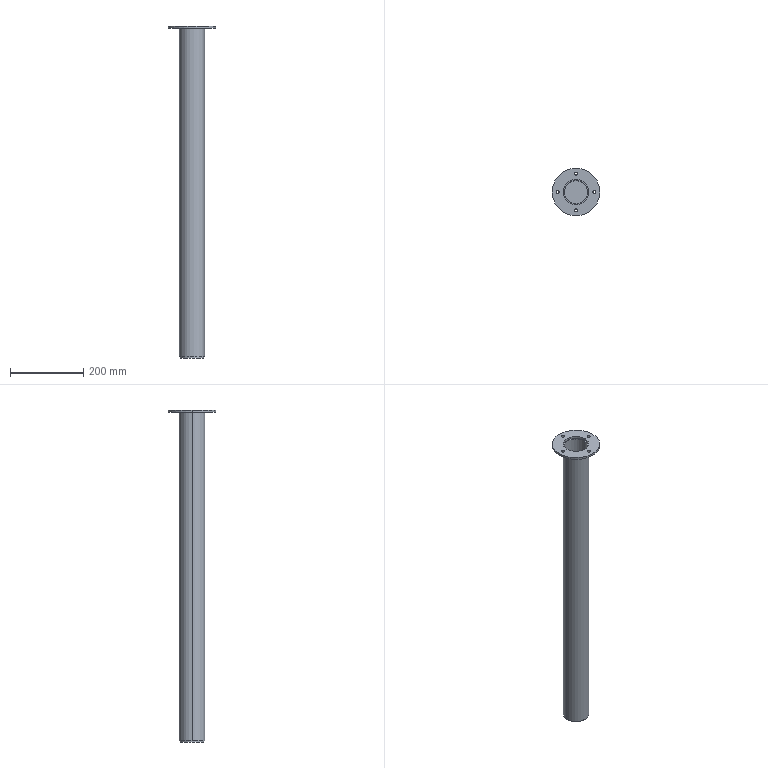Part | SolidWorks | features ICE 2, ExtruThin 1, HoleWzd 1 | 3 solids | 24 faces | box 130 x 130 x 909 mm | volume 633307 mm3 | cylinder 18 | plane 6 | commonest cylinder face diameters 8 x8 64 x4 70 x4 130 x2
STEP:
#1=CARTESIAN_POINT('',(-32.,0.,900.));
#2=VERTEX_POINT('',#1);
#3=CARTESIAN_POINT('',(32.,0.,900.));
#4=VERTEX_POINT('',#3);
#5=CARTESIAN_POINT('',(0.,0.,900.));
#6=DIRECTION('',(0.,0.,1.));
#7=DIRECTION('',(1.,0.,0.));
#8=AXIS2_PLACEMENT_3D('',#5,#6,#7);
#9=CIRCLE('',#8,32.);
#10=EDGE_CURVE('',#2,#4,#9,.T.);
#11=ORIENTED_EDGE('',*,*,#10,.T.);
#12=CARTESIAN_POINT('',(32.,0.,0.));
#13=VERTEX_POINT('',#12);
#14=CARTESIAN_POINT('',(32.,0.,900.));
#15=DIRECTION('',(0.,0.,-1.));
#16=VECTOR('',#15,1000.);
#17=LINE('',#14,#16);
#18=EDGE_CURVE('',#4,#13,#17,.T.);
#19=ORIENTED_EDGE('',*,*,#18,.T.);
#20=CARTESIAN_POINT('',(-32.,0.,0.));
#21=VERTEX_POINT('',#20);
#22=CARTESIAN_POINT('',(0.,0.,0.));
#23=DIRECTION('',(0.,0.,1.));
#24=DIRECTION('',(1.,0.,0.));
#25=AXIS2_PLACEMENT_3D('',#22,#23,#24);
#26=CIRCLE('',#25,32.);
#27=EDGE_CURVE('',#21,#13,#26,.T.);
#28=ORIENTED_EDGE('',*,*,#27,.F.);
#29=CARTESIAN_POINT('',(-32.,0.,900.));
#30=DIRECTION('',(0.,0.,-1.));
#31=VECTOR('',#30,1000.);
#32=LINE('',#29,#31);
#33=EDGE_CURVE('',#2,#21,#32,.T.);
#34=ORIENTED_EDGE('',*,*,#33,.F.);
#35=EDGE_LOOP('',(#11,#19,#28,#34));
#36=FACE_OUTER_BOUND('',#35,.T.);
#37=CARTESIAN_POINT('',(0.,0.,900.));
#38=DIRECTION('',(0.,0.,-1.));
#39=DIRECTION('',(-1.,0.,0.));
#40=AXIS2_PLACEMENT_3D('',#37,#38,#39);
#41=CYLINDRICAL_SURFACE('',#40,32.);
#42=ADVANCED_FACE('',(#36),#41,.F.);
#43=CARTESIAN_POINT('',(35.,0.,900.));
#44=VERTEX_POINT('',#43);
#45=CARTESIAN_POINT('',(-35.,0.,900.));
#46=VERTEX_POINT('',#45);
#47=CARTESIAN_POINT('',(0.,0.,900.));
#48=DIRECTION('',(0.,0.,1.));
#49=DIRECTION('',(1.,0.,0.));
#50=AXIS2_PLACEMENT_3D('',#47,#48,#49);
#51=CIRCLE('',#50,35.);
#52=EDGE_CURVE('',#44,#46,#51,.T.);
#53=ORIENTED_EDGE('',*,*,#52,.F.);
#54=CARTESIAN_POINT('',(35.,0.,0.));
#55=VERTEX_POINT('',#54);
#56=CARTESIAN_POINT('',(35.,0.,900.));
#57=DIRECTION('',(0.,0.,-1.));
#58=VECTOR('',#57,1000.);
#59=LINE('',#56,#58);
#60=EDGE_CURVE('',#44,#55,#59,.T.);
#61=ORIENTED_EDGE('',*,*,#60,.T.);
#62=CARTESIAN_POINT('',(-35.,0.,0.));
#63=VERTEX_POINT('',#62);
#64=CARTESIAN_POINT('',(0.,0.,0.));
#65=DIRECTION('',(0.,0.,1.));
#66=DIRECTION('',(1.,0.,0.));
#67=AXIS2_PLACEMENT_3D('',#64,#65,#66);
#68=CIRCLE('',#67,35.);
#69=EDGE_CURVE('',#55,#63,#68,.T.);
#70=ORIENTED_EDGE('',*,*,#69,.T.);
#71=CARTESIAN_POINT('',(-35.,0.,900.));
#72=DIRECTION('',(0.,0.,-1.));
#73=VECTOR('',#72,1000.);
#74=LINE('',#71,#73);
#75=EDGE_CURVE('',#46,#63,#74,.T.);
#76=ORIENTED_EDGE('',*,*,#75,.F.);
#77=EDGE_LOOP('',(#53,#61,#70,#76));
#78=FACE_OUTER_BOUND('',#77,.T.);
#79=CARTESIAN_POINT('',(0.,0.,900.));
#80=DIRECTION('',(0.,0.,-1.));
#81=DIRECTION('',(-1.,0.,0.));
#82=AXIS2_PLACEMENT_3D('',#79,#80,#81);
#83=CYLINDRICAL_SURFACE('',#82,35.);
#84=ADVANCED_FACE('',(#78),#83,.T.);
#85=CARTESIAN_POINT('',(0.,0.,900.));
#86=DIRECTION('',(0.,0.,1.));
#87=DIRECTION('',(1.,0.,0.));
#88=AXIS2_PLACEMENT_3D('',#85,#86,#87);
#89=CIRCLE('',#88,35.);
#90=EDGE_CURVE('',#46,#44,#89,.T.);
#91=ORIENTED_EDGE('',*,*,#90,.T.);
#92=ORIENTED_EDGE('',*,*,#52,.T.);
#93=EDGE_LOOP('',(#91,#92));
#94=FACE_OUTER_BOUND('',#93,.T.);
#95=ORIENTED_EDGE('',*,*,#10,.F.);
#96=CARTESIAN_POINT('',(0.,0.,900.));
#97=DIRECTION('',(0.,0.,1.));
#98=DIRECTION('',(1.,0.,0.));
#99=AXIS2_PLACEMENT_3D('',#96,#97,#98);
#100=CIRCLE('',#99,32.);
#101=EDGE_CURVE('',#4,#2,#100,.T.);
#102=ORIENTED_EDGE('',*,*,#101,.F.);
#103=EDGE_LOOP('',(#95,#102));
#104=FACE_BOUND('',#103,.T.);
#105=CARTESIAN_POINT('',(0.,0.,900.));
#106=DIRECTION('',(0.,0.,1.));
#107=DIRECTION('',(1.,0.,0.));
#108=AXIS2_PLACEMENT_3D('',#105,#106,#107);
#109=PLANE('',#108);
#110=ADVANCED_FACE('',(#94,#104),#109,.T.);
#111=CARTESIAN_POINT('',(0.,0.,0.));
#112=DIRECTION('',(0.,0.,1.));
#113=DIRECTION('',(1.,0.,0.));
#114=AXIS2_PLACEMENT_3D('',#111,#112,#113);
#115=CIRCLE('',#114,35.);
#116=EDGE_CURVE('',#63,#55,#115,.T.);
#117=ORIENTED_EDGE('',*,*,#116,.F.);
#118=ORIENTED_EDGE('',*,*,#69,.F.);
#119=EDGE_LOOP('',(#117,#118));
#120=FACE_OUTER_BOUND('',#119,.T.);
#121=ORIENTED_EDGE('',*,*,#27,.T.);
#122=CARTESIAN_POINT('',(0.,0.,0.));
#123=DIRECTION('',(0.,0.,1.));
#124=DIRECTION('',(1.,0.,0.));
#125=AXIS2_PLACEMENT_3D('',#122,#123,#124);
#126=CIRCLE('',#125,32.);
#127=EDGE_CURVE('',#13,#21,#126,.T.);
#128=ORIENTED_EDGE('',*,*,#127,.T.);
#129=EDGE_LOOP('',(#121,#128));
#130=FACE_BOUND('',#129,.T.);
#131=CARTESIAN_POINT('',(0.,0.,0.));
#132=DIRECTION('',(0.,0.,1.));
#133=DIRECTION('',(1.,0.,0.));
#134=AXIS2_PLACEMENT_3D('',#131,#132,#133);
#135=PLANE('',#134);
#136=ADVANCED_FACE('',(#120,#130),#135,.F.);
#137=ORIENTED_EDGE('',*,*,#60,.F.);
#138=ORIENTED_EDGE('',*,*,#90,.F.);
#139=ORIENTED_EDGE('',*,*,#75,.T.);
#140=ORIENTED_EDGE('',*,*,#116,.T.);
#141=EDGE_LOOP('',(#137,#138,#139,#140));
#142=FACE_OUTER_BOUND('',#141,.T.);
#143=CARTESIAN_POINT('',(0.,0.,900.));
#144=DIRECTION('',(0.,0.,-1.));
#145=DIRECTION('',(-1.,0.,0.));
#146=AXIS2_PLACEMENT_3D('',#143,#144,#145);
#147=CYLINDRICAL_SURFACE('',#146,35.);
#148=ADVANCED_FACE('',(#142),#147,.T.);
#149=ORIENTED_EDGE('',*,*,#18,.F.);
#150=ORIENTED_EDGE('',*,*,#101,.T.);
#151=ORIENTED_EDGE('',*,*,#33,.T.);
#152=ORIENTED_EDGE('',*,*,#127,.F.);
#153=EDGE_LOOP('',(#149,#150,#151,#152));
#154=FACE_OUTER_BOUND('',#153,.T.);
#155=CARTESIAN_POINT('',(0.,0.,900.));
#156=DIRECTION('',(0.,0.,-1.));
#157=DIRECTION('',(-1.,0.,0.));
#158=AXIS2_PLACEMENT_3D('',#155,#156,#157);
#159=CYLINDRICAL_SURFACE('',#158,32.);
#160=ADVANCED_FACE('',(#154),#159,.F.);
#161=CLOSED_SHELL('',(#42,#84,#110,#136,#148,#160));
#162=MANIFOLD_SOLID_BREP('',#161);
#163=CARTESIAN_POINT('',(-32.,0.,-3.));
#164=VERTEX_POINT('',#163);
#165=CARTESIAN_POINT('',(32.,0.,-3.));
#166=VERTEX_POINT('',#165);
#167=CARTESIAN_POINT('',(0.,0.,-3.));
#168=DIRECTION('',(0.,0.,-1.));
#169=DIRECTION('',(-1.,0.,0.));
#170=AXIS2_PLACEMENT_3D('',#167,#168,#169);
#171=CIRCLE('',#170,32.);
#172=EDGE_CURVE('',#164,#166,#171,.T.);
#173=ORIENTED_EDGE('',*,*,#172,.F.);
#174=CARTESIAN_POINT('',(-32.,0.,0.));
#175=VERTEX_POINT('',#174);
#176=CARTESIAN_POINT('',(-32.,0.,-3.));
#177=DIRECTION('',(0.,0.,1.));
#178=VECTOR('',#177,1000.);
#179=LINE('',#176,#178);
#180=EDGE_CURVE('',#164,#175,#179,.T.);
#181=ORIENTED_EDGE('',*,*,#180,.T.);
#182=CARTESIAN_POINT('',(32.,0.,0.));
#183=VERTEX_POINT('',#182);
#184=CARTESIAN_POINT('',(0.,0.,0.));
#185=DIRECTION('',(0.,0.,-1.));
#186=DIRECTION('',(-1.,0.,0.));
#187=AXIS2_PLACEMENT_3D('',#184,#185,#186);
#188=CIRCLE('',#187,32.);
#189=EDGE_CURVE('',#175,#183,#188,.T.);
#190=ORIENTED_EDGE('',*,*,#189,.T.);
#191=CARTESIAN_POINT('',(32.,0.,-3.));
#192=DIRECTION('',(0.,0.,1.));
#193=VECTOR('',#192,1000.);
#194=LINE('',#191,#193);
#195=EDGE_CURVE('',#166,#183,#194,.T.);
#196=ORIENTED_EDGE('',*,*,#195,.F.);
#197=EDGE_LOOP('',(#173,#181,#190,#196));
#198=FACE_OUTER_BOUND('',#197,.T.);
#199=CARTESIAN_POINT('',(0.,0.,-3.));
#200=DIRECTION('',(0.,0.,1.));
#201=DIRECTION('',(1.,0.,0.));
#202=AXIS2_PLACEMENT_3D('',#199,#200,#201);
#203=CYLINDRICAL_SURFACE('',#202,32.);
#204=ADVANCED_FACE('',(#198),#203,.T.);
#205=ORIENTED_EDGE('',*,*,#180,.F.);
#206=CARTESIAN_POINT('',(0.,0.,-3.));
#207=DIRECTION('',(0.,0.,-1.));
#208=DIRECTION('',(-1.,0.,0.));
#209=AXIS2_PLACEMENT_3D('',#206,#207,#208);
#210=CIRCLE('',#209,32.);
#211=EDGE_CURVE('',#166,#164,#210,.T.);
#212=ORIENTED_EDGE('',*,*,#211,.F.);
#213=ORIENTED_EDGE('',*,*,#195,.T.);
#214=CARTESIAN_POINT('',(0.,0.,0.));
#215=DIRECTION('',(0.,0.,-1.));
#216=DIRECTION('',(-1.,0.,0.));
#217=AXIS2_PLACEMENT_3D('',#214,#215,#216);
#218=CIRCLE('',#217,32.);
#219=EDGE_CURVE('',#183,#175,#218,.T.);
#220=ORIENTED_EDGE('',*,*,#219,.T.);
#221=EDGE_LOOP('',(#205,#212,#213,#220));
#222=FACE_OUTER_BOUND('',#221,.T.);
#223=CARTESIAN_POINT('',(0.,0.,-3.));
#224=DIRECTION('',(0.,0.,1.));
#225=DIRECTION('',(1.,0.,0.));
#226=AXIS2_PLACEMENT_3D('',#223,#224,#225);
#227=CYLINDRICAL_SURFACE('',#226,32.);
#228=ADVANCED_FACE('',(#222),#227,.T.);
#229=ORIENTED_EDGE('',*,*,#211,.T.);
#230=ORIENTED_EDGE('',*,*,#172,.T.);
#231=EDGE_LOOP('',(#229,#230));
#232=FACE_OUTER_BOUND('',#231,.T.);
#233=CARTESIAN_POINT('',(0.,0.,-3.));
#234=DIRECTION('',(0.,0.,-1.));
#235=DIRECTION('',(-1.,0.,0.));
#236=AXIS2_PLACEMENT_3D('',#233,#234,#235);
#237=PLANE('',#236);
#238=ADVANCED_FACE('',(#232),#237,.T.);
#239=ORIENTED_EDGE('',*,*,#219,.F.);
#240=ORIENTED_EDGE('',*,*,#189,.F.);
#241=EDGE_LOOP('',(#239,#240));
#242=FACE_OUTER_BOUND('',#241,.T.);
#243=CARTESIAN_POINT('',(0.,0.,0.));
#244=DIRECTION('',(0.,0.,-1.));
#245=DIRECTION('',(-1.,0.,0.));
#246=AXIS2_PLACEMENT_3D('',#243,#244,#245);
#247=PLANE('',#246);
#248=ADVANCED_FACE('',(#242),#247,.F.);
#249=CLOSED_SHELL('',(#204,#228,#238,#248));
#250=MANIFOLD_SOLID_BREP('',#249);
#251=CARTESIAN_POINT('',(-4.,50.,900.));
#252=VERTEX_POINT('',#251);
#253=CARTESIAN_POINT('',(4.,50.,900.));
#254=VERTEX_POINT('',#253);
#255=CARTESIAN_POINT('',(0.,50.,900.));
#256=DIRECTION('',(0.,0.,1.));
#257=DIRECTION('',(1.,0.,0.));
#258=AXIS2_PLACEMENT_3D('',#255,#256,#257);
#259=CIRCLE('',#258,4.);
#260=EDGE_CURVE('',#252,#254,#259,.T.);
#261=ORIENTED_EDGE('',*,*,#260,.F.);
#262=CARTESIAN_POINT('',(-4.,50.,906.));
#263=VERTEX_POINT('',#262);
#264=CARTESIAN_POINT('',(-4.,50.,906.));
#265=DIRECTION('',(0.,0.,1.));
#266=VECTOR('',#265,1000.);
#267=LINE('',#264,#266);
#268=EDGE_CURVE('',#252,#263,#267,.T.);
#269=ORIENTED_EDGE('',*,*,#268,.T.);
#270=CARTESIAN_POINT('',(4.,50.,906.));
#271=VERTEX_POINT('',#270);
#272=CARTESIAN_POINT('',(0.,50.,906.));
#273=DIRECTION('',(0.,0.,1.));
#274=DIRECTION('',(1.,0.,0.));
#275=AXIS2_PLACEMENT_3D('',#272,#273,#274);
#276=CIRCLE('',#275,4.);
#277=EDGE_CURVE('',#263,#271,#276,.T.);
#278=ORIENTED_EDGE('',*,*,#277,.T.);
#279=CARTESIAN_POINT('',(4.,50.,906.));
#280=DIRECTION('',(0.,0.,1.));
#281=VECTOR('',#280,1000.);
#282=LINE('',#279,#281);
#283=EDGE_CURVE('',#254,#271,#282,.T.);
#284=ORIENTED_EDGE('',*,*,#283,.F.);
#285=EDGE_LOOP('',(#261,#269,#278,#284));
#286=FACE_OUTER_BOUND('',#285,.T.);
#287=CARTESIAN_POINT('',(0.,50.,906.));
#288=DIRECTION('',(0.,0.,1.));
#289=DIRECTION('',(1.,0.,0.));
#290=AXIS2_PLACEMENT_3D('',#287,#288,#289);
#291=CYLINDRICAL_SURFACE('',#290,4.);
#292=ADVANCED_FACE('',(#286),#291,.F.);
#293=CARTESIAN_POINT('',(-54.,0.,900.));
#294=VERTEX_POINT('',#293);
#295=CARTESIAN_POINT('',(-46.,0.,900.));
#296=VERTEX_POINT('',#295);
#297=CARTESIAN_POINT('',(-50.,0.,900.));
#298=DIRECTION('',(0.,0.,1.));
#299=DIRECTION('',(1.,0.,0.));
#300=AXIS2_PLACEMENT_3D('',#297,#298,#299);
#301=CIRCLE('',#300,4.);
#302=EDGE_CURVE('',#294,#296,#301,.T.);
#303=ORIENTED_EDGE('',*,*,#302,.F.);
#304=CARTESIAN_POINT('',(-54.,0.,906.));
#305=VERTEX_POINT('',#304);
#306=CARTESIAN_POINT('',(-54.,0.,906.));
#307=DIRECTION('',(0.,0.,1.));
#308=VECTOR('',#307,1000.);
#309=LINE('',#306,#308);
#310=EDGE_CURVE('',#294,#305,#309,.T.);
#311=ORIENTED_EDGE('',*,*,#310,.T.);
#312=CARTESIAN_POINT('',(-46.,0.,906.));
#313=VERTEX_POINT('',#312);
#314=CARTESIAN_POINT('',(-50.,0.,906.));
#315=DIRECTION('',(0.,0.,1.));
#316=DIRECTION('',(1.,0.,0.));
#317=AXIS2_PLACEMENT_3D('',#314,#315,#316);
#318=CIRCLE('',#317,4.);
#319=EDGE_CURVE('',#305,#313,#318,.T.);
#320=ORIENTED_EDGE('',*,*,#319,.T.);
#321=CARTESIAN_POINT('',(-46.,0.,906.));
#322=DIRECTION('',(0.,0.,1.));
#323=VECTOR('',#322,1000.);
#324=LINE('',#321,#323);
#325=EDGE_CURVE('',#296,#313,#324,.T.);
#326=ORIENTED_EDGE('',*,*,#325,.F.);
#327=EDGE_LOOP('',(#303,#311,#320,#326));
#328=FACE_OUTER_BOUND('',#327,.T.);
#329=CARTESIAN_POINT('',(-50.,0.,906.));
#330=DIRECTION('',(0.,0.,1.));
#331=DIRECTION('',(1.,0.,0.));
#332=AXIS2_PLACEMENT_3D('',#329,#330,#331);
#333=CYLINDRICAL_SURFACE('',#332,4.);
#334=ADVANCED_FACE('',(#328),#333,.F.);
#335=CARTESIAN_POINT('',(-4.,-50.,900.));
#336=VERTEX_POINT('',#335);
#337=CARTESIAN_POINT('',(4.,-50.,900.));
#338=VERTEX_POINT('',#337);
#339=CARTESIAN_POINT('',(0.,-50.,900.));
#340=DIRECTION('',(0.,0.,1.));
#341=DIRECTION('',(1.,0.,0.));
#342=AXIS2_PLACEMENT_3D('',#339,#340,#341);
#343=CIRCLE('',#342,4.);
#344=EDGE_CURVE('',#336,#338,#343,.T.);
#345=ORIENTED_EDGE('',*,*,#344,.F.);
#346=CARTESIAN_POINT('',(-4.,-50.,906.));
#347=VERTEX_POINT('',#346);
#348=CARTESIAN_POINT('',(-4.,-50.,906.));
#349=DIRECTION('',(0.,0.,1.));
#350=VECTOR('',#349,1000.);
#351=LINE('',#348,#350);
#352=EDGE_CURVE('',#336,#347,#351,.T.);
#353=ORIENTED_EDGE('',*,*,#352,.T.);
#354=CARTESIAN_POINT('',(4.,-50.,906.));
#355=VERTEX_POINT('',#354);
#356=CARTESIAN_POINT('',(0.,-50.,906.));
#357=DIRECTION('',(0.,0.,1.));
#358=DIRECTION('',(1.,0.,0.));
#359=AXIS2_PLACEMENT_3D('',#356,#357,#358);
#360=CIRCLE('',#359,4.);
#361=EDGE_CURVE('',#347,#355,#360,.T.);
#362=ORIENTED_EDGE('',*,*,#361,.T.);
#363=CARTESIAN_POINT('',(4.,-50.,906.));
#364=DIRECTION('',(0.,0.,1.));
#365=VECTOR('',#364,1000.);
#366=LINE('',#363,#365);
#367=EDGE_CURVE('',#338,#355,#366,.T.);
#368=ORIENTED_EDGE('',*,*,#367,.F.);
#369=EDGE_LOOP('',(#345,#353,#362,#368));
#370=FACE_OUTER_BOUND('',#369,.T.);
#371=CARTESIAN_POINT('',(0.,-50.,906.));
#372=DIRECTION('',(0.,0.,1.));
#373=DIRECTION('',(1.,0.,0.));
#374=AXIS2_PLACEMENT_3D('',#371,#372,#373);
#375=CYLINDRICAL_SURFACE('',#374,4.);
#376=ADVANCED_FACE('',(#370),#375,.F.);
#377=CARTESIAN_POINT('',(46.,0.,900.));
#378=VERTEX_POINT('',#377);
#379=CARTESIAN_POINT('',(54.,0.,900.));
#380=VERTEX_POINT('',#379);
#381=CARTESIAN_POINT('',(50.,0.,900.));
#382=DIRECTION('',(0.,0.,1.));
#383=DIRECTION('',(1.,0.,0.));
#384=AXIS2_PLACEMENT_3D('',#381,#382,#383);
#385=CIRCLE('',#384,4.);
#386=EDGE_CURVE('',#378,#380,#385,.T.);
#387=ORIENTED_EDGE('',*,*,#386,.F.);
#388=CARTESIAN_POINT('',(46.,0.,906.));
#389=VERTEX_POINT('',#388);
#390=CARTESIAN_POINT('',(46.,0.,906.));
#391=DIRECTION('',(0.,0.,1.));
#392=VECTOR('',#391,1000.);
#393=LINE('',#390,#392);
#394=EDGE_CURVE('',#378,#389,#393,.T.);
#395=ORIENTED_EDGE('',*,*,#394,.T.);
#396=CARTESIAN_POINT('',(54.,0.,906.));
#397=VERTEX_POINT('',#396);
#398=CARTESIAN_POINT('',(50.,0.,906.));
#399=DIRECTION('',(0.,0.,1.));
#400=DIRECTION('',(1.,0.,0.));
#401=AXIS2_PLACEMENT_3D('',#398,#399,#400);
#402=CIRCLE('',#401,4.);
#403=EDGE_CURVE('',#389,#397,#402,.T.);
#404=ORIENTED_EDGE('',*,*,#403,.T.);
#405=CARTESIAN_POINT('',(54.,0.,906.));
#406=DIRECTION('',(0.,0.,1.));
#407=VECTOR('',#406,1000.);
#408=LINE('',#405,#407);
#409=EDGE_CURVE('',#380,#397,#408,.T.);
#410=ORIENTED_EDGE('',*,*,#409,.F.);
#411=EDGE_LOOP('',(#387,#395,#404,#410));
#412=FACE_OUTER_BOUND('',#411,.T.);
#413=CARTESIAN_POINT('',(50.,0.,906.));
#414=DIRECTION('',(0.,0.,1.));
#415=DIRECTION('',(1.,0.,0.));
#416=AXIS2_PLACEMENT_3D('',#413,#414,#415);
#417=CYLINDRICAL_SURFACE('',#416,4.);
#418=ADVANCED_FACE('',(#412),#417,.F.);
#419=CARTESIAN_POINT('',(-35.,0.,906.));
#420=VERTEX_POINT('',#419);
#421=CARTESIAN_POINT('',(35.,0.,906.));
#422=VERTEX_POINT('',#421);
#423=CARTESIAN_POINT('',(0.,0.,906.));
#424=DIRECTION('',(0.,0.,1.));
#425=DIRECTION('',(1.,0.,0.));
#426=AXIS2_PLACEMENT_3D('',#423,#424,#425);
#427=CIRCLE('',#426,35.);
#428=EDGE_CURVE('',#420,#422,#427,.T.);
#429=ORIENTED_EDGE('',*,*,#428,.T.);
#430=CARTESIAN_POINT('',(35.,0.,900.));
#431=VERTEX_POINT('',#430);
#432=CARTESIAN_POINT('',(35.,0.,906.));
#433=DIRECTION('',(0.,0.,-1.));
#434=VECTOR('',#433,1000.);
#435=LINE('',#432,#434);
#436=EDGE_CURVE('',#422,#431,#435,.T.);
#437=ORIENTED_EDGE('',*,*,#436,.T.);
#438=CARTESIAN_POINT('',(-35.,0.,900.));
#439=VERTEX_POINT('',#438);
#440=CARTESIAN_POINT('',(0.,0.,900.));
#441=DIRECTION('',(0.,0.,1.));
#442=DIRECTION('',(1.,0.,0.));
#443=AXIS2_PLACEMENT_3D('',#440,#441,#442);
#444=CIRCLE('',#443,35.);
#445=EDGE_CURVE('',#439,#431,#444,.T.);
#446=ORIENTED_EDGE('',*,*,#445,.F.);
#447=CARTESIAN_POINT('',(-35.,0.,906.));
#448=DIRECTION('',(0.,0.,-1.));
#449=VECTOR('',#448,1000.);
#450=LINE('',#447,#449);
#451=EDGE_CURVE('',#420,#439,#450,.T.);
#452=ORIENTED_EDGE('',*,*,#451,.F.);
#453=EDGE_LOOP('',(#429,#437,#446,#452));
#454=FACE_OUTER_BOUND('',#453,.T.);
#455=CARTESIAN_POINT('',(0.,0.,906.));
#456=DIRECTION('',(0.,0.,-1.));
#457=DIRECTION('',(-1.,0.,0.));
#458=AXIS2_PLACEMENT_3D('',#455,#456,#457);
#459=CYLINDRICAL_SURFACE('',#458,35.);
#460=ADVANCED_FACE('',(#454),#459,.F.);
#461=CARTESIAN_POINT('',(65.,0.,906.));
#462=VERTEX_POINT('',#461);
#463=CARTESIAN_POINT('',(-65.,0.,906.));
#464=VERTEX_POINT('',#463);
#465=CARTESIAN_POINT('',(0.,0.,906.));
#466=DIRECTION('',(0.,0.,1.));
#467=DIRECTION('',(1.,0.,0.));
#468=AXIS2_PLACEMENT_3D('',#465,#466,#467);
#469=CIRCLE('',#468,65.);
#470=EDGE_CURVE('',#462,#464,#469,.T.);
#471=ORIENTED_EDGE('',*,*,#470,.F.);
#472=CARTESIAN_POINT('',(65.,0.,900.));
#473=VERTEX_POINT('',#472);
#474=CARTESIAN_POINT('',(65.,0.,906.));
#475=DIRECTION('',(0.,0.,-1.));
#476=VECTOR('',#475,1000.);
#477=LINE('',#474,#476);
#478=EDGE_CURVE('',#462,#473,#477,.T.);
#479=ORIENTED_EDGE('',*,*,#478,.T.);
#480=CARTESIAN_POINT('',(-65.,0.,900.));
#481=VERTEX_POINT('',#480);
#482=CARTESIAN_POINT('',(0.,0.,900.));
#483=DIRECTION('',(0.,0.,1.));
#484=DIRECTION('',(1.,0.,0.));
#485=AXIS2_PLACEMENT_3D('',#482,#483,#484);
#486=CIRCLE('',#485,65.);
#487=EDGE_CURVE('',#473,#481,#486,.T.);
#488=ORIENTED_EDGE('',*,*,#487,.T.);
#489=CARTESIAN_POINT('',(-65.,0.,906.));
#490=DIRECTION('',(0.,0.,-1.));
#491=VECTOR('',#490,1000.);
#492=LINE('',#489,#491);
#493=EDGE_CURVE('',#464,#481,#492,.T.);
#494=ORIENTED_EDGE('',*,*,#493,.F.);
#495=EDGE_LOOP('',(#471,#479,#488,#494));
#496=FACE_OUTER_BOUND('',#495,.T.);
#497=CARTESIAN_POINT('',(0.,0.,906.));
#498=DIRECTION('',(0.,0.,-1.));
#499=DIRECTION('',(-1.,0.,0.));
#500=AXIS2_PLACEMENT_3D('',#497,#498,#499);
#501=CYLINDRICAL_SURFACE('',#500,65.);
#502=ADVANCED_FACE('',(#496),#501,.T.);
#503=CARTESIAN_POINT('',(0.,50.,906.));
#504=DIRECTION('',(0.,0.,1.));
#505=DIRECTION('',(1.,0.,0.));
#506=AXIS2_PLACEMENT_3D('',#503,#504,#505);
#507=CIRCLE('',#506,4.);
#508=EDGE_CURVE('',#271,#263,#507,.T.);
#509=ORIENTED_EDGE('',*,*,#508,.F.);
#510=ORIENTED_EDGE('',*,*,#277,.F.);
#511=EDGE_LOOP('',(#509,#510));
#512=FACE_BOUND('',#511,.T.);
#513=CARTESIAN_POINT('',(-50.,0.,906.));
#514=DIRECTION('',(0.,0.,1.));
#515=DIRECTION('',(1.,0.,0.));
#516=AXIS2_PLACEMENT_3D('',#513,#514,#515);
#517=CIRCLE('',#516,4.);
#518=EDGE_CURVE('',#313,#305,#517,.T.);
#519=ORIENTED_EDGE('',*,*,#518,.F.);
#520=ORIENTED_EDGE('',*,*,#319,.F.);
#521=EDGE_LOOP('',(#519,#520));
#522=FACE_BOUND('',#521,.T.);
#523=CARTESIAN_POINT('',(0.,-50.,906.));
#524=DIRECTION('',(0.,0.,1.));
#525=DIRECTION('',(1.,0.,0.));
#526=AXIS2_PLACEMENT_3D('',#523,#524,#525);
#527=CIRCLE('',#526,4.);
#528=EDGE_CURVE('',#355,#347,#527,.T.);
#529=ORIENTED_EDGE('',*,*,#528,.F.);
#530=ORIENTED_EDGE('',*,*,#361,.F.);
#531=EDGE_LOOP('',(#529,#530));
#532=FACE_BOUND('',#531,.T.);
#533=CARTESIAN_POINT('',(50.,0.,906.));
#534=DIRECTION('',(0.,0.,1.));
#535=DIRECTION('',(1.,0.,0.));
#536=AXIS2_PLACEMENT_3D('',#533,#534,#535);
#537=CIRCLE('',#536,4.);
#538=EDGE_CURVE('',#397,#389,#537,.T.);
#539=ORIENTED_EDGE('',*,*,#538,.F.);
#540=ORIENTED_EDGE('',*,*,#403,.F.);
#541=EDGE_LOOP('',(#539,#540));
#542=FACE_BOUND('',#541,.T.);
#543=CARTESIAN_POINT('',(0.,0.,906.));
#544=DIRECTION('',(0.,0.,1.));
#545=DIRECTION('',(1.,0.,0.));
#546=AXIS2_PLACEMENT_3D('',#543,#544,#545);
#547=CIRCLE('',#546,65.);
#548=EDGE_CURVE('',#464,#462,#547,.T.);
#549=ORIENTED_EDGE('',*,*,#548,.T.);
#550=ORIENTED_EDGE('',*,*,#470,.T.);
#551=EDGE_LOOP('',(#549,#550));
#552=FACE_OUTER_BOUND('',#551,.T.);
#553=ORIENTED_EDGE('',*,*,#428,.F.);
#554=CARTESIAN_POINT('',(0.,0.,906.));
#555=DIRECTION('',(0.,0.,1.));
#556=DIRECTION('',(1.,0.,0.));
#557=AXIS2_PLACEMENT_3D('',#554,#555,#556);
#558=CIRCLE('',#557,35.);
#559=EDGE_CURVE('',#422,#420,#558,.T.);
#560=ORIENTED_EDGE('',*,*,#559,.F.);
#561=EDGE_LOOP('',(#553,#560));
#562=FACE_BOUND('',#561,.T.);
#563=CARTESIAN_POINT('',(0.,0.,906.));
#564=DIRECTION('',(0.,0.,1.));
#565=DIRECTION('',(1.,0.,0.));
#566=AXIS2_PLACEMENT_3D('',#563,#564,#565);
#567=PLANE('',#566);
#568=ADVANCED_FACE('',(#512,#522,#532,#542,#552,#562),#567,.T.);
#569=CARTESIAN_POINT('',(0.,50.,900.));
#570=DIRECTION('',(0.,0.,1.));
#571=DIRECTION('',(1.,0.,0.));
#572=AXIS2_PLACEMENT_3D('',#569,#570,#571);
#573=CIRCLE('',#572,4.);
#574=EDGE_CURVE('',#254,#252,#573,.T.);
#575=ORIENTED_EDGE('',*,*,#574,.T.);
#576=ORIENTED_EDGE('',*,*,#260,.T.);
#577=EDGE_LOOP('',(#575,#576));
#578=FACE_BOUND('',#577,.T.);
#579=CARTESIAN_POINT('',(-50.,0.,900.));
#580=DIRECTION('',(0.,0.,1.));
#581=DIRECTION('',(1.,0.,0.));
#582=AXIS2_PLACEMENT_3D('',#579,#580,#581);
#583=CIRCLE('',#582,4.);
#584=EDGE_CURVE('',#296,#294,#583,.T.);
#585=ORIENTED_EDGE('',*,*,#584,.T.);
#586=ORIENTED_EDGE('',*,*,#302,.T.);
#587=EDGE_LOOP('',(#585,#586));
#588=FACE_BOUND('',#587,.T.);
#589=CARTESIAN_POINT('',(0.,-50.,900.));
#590=DIRECTION('',(0.,0.,1.));
#591=DIRECTION('',(1.,0.,0.));
#592=AXIS2_PLACEMENT_3D('',#589,#590,#591);
#593=CIRCLE('',#592,4.);
#594=EDGE_CURVE('',#338,#336,#593,.T.);
#595=ORIENTED_EDGE('',*,*,#594,.T.);
#596=ORIENTED_EDGE('',*,*,#344,.T.);
#597=EDGE_LOOP('',(#595,#596));
#598=FACE_BOUND('',#597,.T.);
#599=CARTESIAN_POINT('',(50.,0.,900.));
#600=DIRECTION('',(0.,0.,1.));
#601=DIRECTION('',(1.,0.,0.));
#602=AXIS2_PLACEMENT_3D('',#599,#600,#601);
#603=CIRCLE('',#602,4.);
#604=EDGE_CURVE('',#380,#378,#603,.T.);
#605=ORIENTED_EDGE('',*,*,#604,.T.);
#606=ORIENTED_EDGE('',*,*,#386,.T.);
#607=EDGE_LOOP('',(#605,#606));
#608=FACE_BOUND('',#607,.T.);
#609=CARTESIAN_POINT('',(0.,0.,900.));
#610=DIRECTION('',(0.,0.,1.));
#611=DIRECTION('',(1.,0.,0.));
#612=AXIS2_PLACEMENT_3D('',#609,#610,#611);
#613=CIRCLE('',#612,65.);
#614=EDGE_CURVE('',#481,#473,#613,.T.);
#615=ORIENTED_EDGE('',*,*,#614,.F.);
#616=ORIENTED_EDGE('',*,*,#487,.F.);
#617=EDGE_LOOP('',(#615,#616));
#618=FACE_OUTER_BOUND('',#617,.T.);
#619=ORIENTED_EDGE('',*,*,#445,.T.);
#620=CARTESIAN_POINT('',(0.,0.,900.));
#621=DIRECTION('',(0.,0.,1.));
#622=DIRECTION('',(1.,0.,0.));
#623=AXIS2_PLACEMENT_3D('',#620,#621,#622);
#624=CIRCLE('',#623,35.);
#625=EDGE_CURVE('',#431,#439,#624,.T.);
#626=ORIENTED_EDGE('',*,*,#625,.T.);
#627=EDGE_LOOP('',(#619,#626));
#628=FACE_BOUND('',#627,.T.);
#629=CARTESIAN_POINT('',(0.,0.,900.));
#630=DIRECTION('',(0.,0.,1.));
#631=DIRECTION('',(1.,0.,0.));
#632=AXIS2_PLACEMENT_3D('',#629,#630,#631);
#633=PLANE('',#632);
#634=ADVANCED_FACE('',(#578,#588,#598,#608,#618,#628),#633,.F.);
#635=ORIENTED_EDGE('',*,*,#478,.F.);
#636=ORIENTED_EDGE('',*,*,#548,.F.);
#637=ORIENTED_EDGE('',*,*,#493,.T.);
#638=ORIENTED_EDGE('',*,*,#614,.T.);
#639=EDGE_LOOP('',(#635,#636,#637,#638));
#640=FACE_OUTER_BOUND('',#639,.T.);
#641=CARTESIAN_POINT('',(0.,0.,906.));
#642=DIRECTION('',(0.,0.,-1.));
#643=DIRECTION('',(-1.,0.,0.));
#644=AXIS2_PLACEMENT_3D('',#641,#642,#643);
#645=CYLINDRICAL_SURFACE('',#644,65.);
#646=ADVANCED_FACE('',(#640),#645,.T.);
#647=ORIENTED_EDGE('',*,*,#436,.F.);
#648=ORIENTED_EDGE('',*,*,#559,.T.);
#649=ORIENTED_EDGE('',*,*,#451,.T.);
#650=ORIENTED_EDGE('',*,*,#625,.F.);
#651=EDGE_LOOP('',(#647,#648,#649,#650));
#652=FACE_OUTER_BOUND('',#651,.T.);
#653=CARTESIAN_POINT('',(0.,0.,906.));
#654=DIRECTION('',(0.,0.,-1.));
#655=DIRECTION('',(-1.,0.,0.));
#656=AXIS2_PLACEMENT_3D('',#653,#654,#655);
#657=CYLINDRICAL_SURFACE('',#656,35.);
#658=ADVANCED_FACE('',(#652),#657,.F.);
#659=ORIENTED_EDGE('',*,*,#394,.F.);
#660=ORIENTED_EDGE('',*,*,#604,.F.);
#661=ORIENTED_EDGE('',*,*,#409,.T.);
#662=ORIENTED_EDGE('',*,*,#538,.T.);
#663=EDGE_LOOP('',(#659,#660,#661,#662));
#664=FACE_OUTER_BOUND('',#663,.T.);
#665=CARTESIAN_POINT('',(50.,0.,906.));
#666=DIRECTION('',(0.,0.,1.));
#667=DIRECTION('',(1.,0.,0.));
#668=AXIS2_PLACEMENT_3D('',#665,#666,#667);
#669=CYLINDRICAL_SURFACE('',#668,4.);
#670=ADVANCED_FACE('',(#664),#669,.F.);
#671=ORIENTED_EDGE('',*,*,#352,.F.);
#672=ORIENTED_EDGE('',*,*,#594,.F.);
#673=ORIENTED_EDGE('',*,*,#367,.T.);
#674=ORIENTED_EDGE('',*,*,#528,.T.);
#675=EDGE_LOOP('',(#671,#672,#673,#674));
#676=FACE_OUTER_BOUND('',#675,.T.);
#677=CARTESIAN_POINT('',(0.,-50.,906.));
#678=DIRECTION('',(0.,0.,1.));
#679=DIRECTION('',(1.,0.,0.));
#680=AXIS2_PLACEMENT_3D('',#677,#678,#679);
#681=CYLINDRICAL_SURFACE('',#680,4.);
#682=ADVANCED_FACE('',(#676),#681,.F.);
#683=ORIENTED_EDGE('',*,*,#310,.F.);
#684=ORIENTED_EDGE('',*,*,#584,.F.);
#685=ORIENTED_EDGE('',*,*,#325,.T.);
#686=ORIENTED_EDGE('',*,*,#518,.T.);
#687=EDGE_LOOP('',(#683,#684,#685,#686));
#688=FACE_OUTER_BOUND('',#687,.T.);
#689=CARTESIAN_POINT('',(-50.,0.,906.));
#690=DIRECTION('',(0.,0.,1.));
#691=DIRECTION('',(1.,0.,0.));
#692=AXIS2_PLACEMENT_3D('',#689,#690,#691);
#693=CYLINDRICAL_SURFACE('',#692,4.);
#694=ADVANCED_FACE('',(#688),#693,.F.);
#695=ORIENTED_EDGE('',*,*,#268,.F.);
#696=ORIENTED_EDGE('',*,*,#574,.F.);
#697=ORIENTED_EDGE('',*,*,#283,.T.);
#698=ORIENTED_EDGE('',*,*,#508,.T.);
#699=EDGE_LOOP('',(#695,#696,#697,#698));
#700=FACE_OUTER_BOUND('',#699,.T.);
#701=CARTESIAN_POINT('',(0.,50.,906.));
#702=DIRECTION('',(0.,0.,1.));
#703=DIRECTION('',(1.,0.,0.));
#704=AXIS2_PLACEMENT_3D('',#701,#702,#703);
#705=CYLINDRICAL_SURFACE('',#704,4.);
#706=ADVANCED_FACE('',(#700),#705,.F.);
#707=CLOSED_SHELL('',(#292,#334,#376,#418,#460,#502,#568,#634,#646,#658,#670,#682,#694,#706));
#708=MANIFOLD_SOLID_BREP('',#707);
#709=CARTESIAN_POINT('',(0.,0.,0.));
#710=DIRECTION('',(0.,0.,1.));
#711=DIRECTION('',(1.,0.,0.));
#712=AXIS2_PLACEMENT_3D('',#709,#710,#711);
#713=(LENGTH_UNIT()NAMED_UNIT(*)SI_UNIT(.MILLI.,.METRE.));
#714=UNCERTAINTY_MEASURE_WITH_UNIT(LENGTH_MEASURE(0.00001),#713,'','');
#715=(NAMED_UNIT(*)PLANE_ANGLE_UNIT()SI_UNIT($,.RADIAN.));
#716=(NAMED_UNIT(*)SI_UNIT($,.STERADIAN.)SOLID_ANGLE_UNIT());
#717=(GEOMETRIC_REPRESENTATION_CONTEXT(3)GLOBAL_UNCERTAINTY_ASSIGNED_CONTEXT((#714))GLOBAL_UNIT_ASSIGNED_CONTEXT((#713,#715,#716))REPRESENTATION_CONTEXT('',''));
#718=ADVANCED_BREP_SHAPE_REPRESENTATION('',(#162,#250,#708,#712),#717);